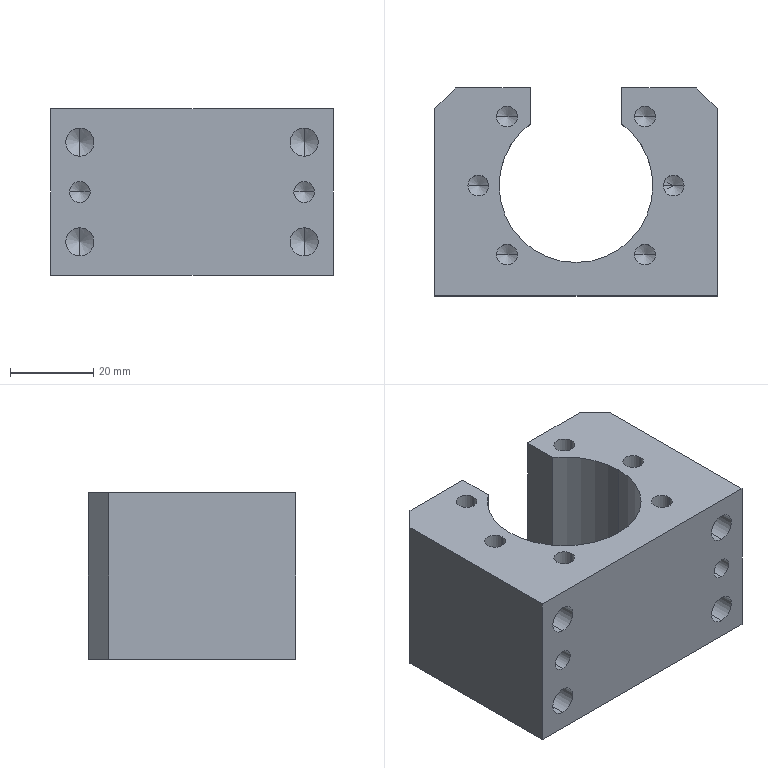Part | SolidWorks | features BaseBody 1 | 1 solid | 70 faces | box 68 x 50 x 40 mm | volume 79325 mm3 | cylinder 31 | cone 28 | plane 11 | commonest cylinder face diameters 5 x16 6.8 x8 10 x4 37 x3